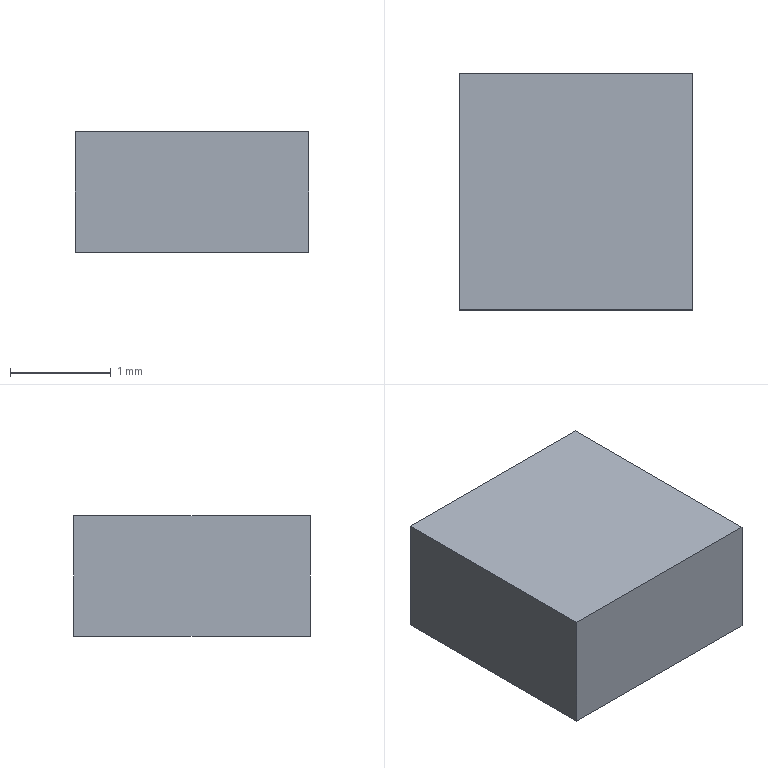Part | Creo | 1 solid | 6 faces | box 2.318 x 2.344 x 1.2 mm | volume 6.521 mm3 | plane 6
STEP:
#1=CARTESIAN_POINT('',(0.,0.,0.));
#2=DIRECTION('',(0.,0.,1.));
#3=DIRECTION('',(1.,0.,0.));
#4=AXIS2_PLACEMENT_3D('',#1,#2,#3);
#5=CARTESIAN_POINT('',(-1.125,-1.125,0.));
#6=VERTEX_POINT('',#5);
#7=CARTESIAN_POINT('',(1.193,-1.125,0.));
#8=VERTEX_POINT('',#7);
#9=CARTESIAN_POINT('',(-1.125,-1.125,0.));
#10=DIRECTION('',(1.,0.,0.));
#11=VECTOR('',#10,2.318);
#12=LINE('',#9,#11);
#13=EDGE_CURVE('',#6,#8,#12,.T.);
#14=ORIENTED_EDGE('',*,*,#13,.T.);
#15=CARTESIAN_POINT('',(1.193,1.219,0.));
#16=VERTEX_POINT('',#15);
#17=CARTESIAN_POINT('',(1.193,-1.125,0.));
#18=DIRECTION('',(0.,1.,0.));
#19=VECTOR('',#18,2.344);
#20=LINE('',#17,#19);
#21=EDGE_CURVE('',#8,#16,#20,.T.);
#22=ORIENTED_EDGE('',*,*,#21,.T.);
#23=CARTESIAN_POINT('',(-1.125,1.219,0.));
#24=VERTEX_POINT('',#23);
#25=CARTESIAN_POINT('',(1.193,1.219,0.));
#26=DIRECTION('',(-1.,0.,0.));
#27=VECTOR('',#26,2.318);
#28=LINE('',#25,#27);
#29=EDGE_CURVE('',#16,#24,#28,.T.);
#30=ORIENTED_EDGE('',*,*,#29,.T.);
#31=CARTESIAN_POINT('',(-1.125,1.219,0.));
#32=DIRECTION('',(0.,-1.,0.));
#33=VECTOR('',#32,2.344);
#34=LINE('',#31,#33);
#35=EDGE_CURVE('',#24,#6,#34,.T.);
#36=ORIENTED_EDGE('',*,*,#35,.T.);
#37=EDGE_LOOP('',(#14,#22,#30,#36));
#38=FACE_OUTER_BOUND('',#37,.F.);
#39=CARTESIAN_POINT('',(0.,0.,0.));
#40=DIRECTION('',(0.,0.,1.));
#41=DIRECTION('',(1.,0.,0.));
#42=AXIS2_PLACEMENT_3D('',#39,#40,#41);
#43=PLANE('',#42);
#44=ADVANCED_FACE('',(#38),#43,.F.);
#45=ORIENTED_EDGE('',*,*,#13,.F.);
#46=CARTESIAN_POINT('',(-1.125,-1.125,1.2));
#47=VERTEX_POINT('',#46);
#48=CARTESIAN_POINT('',(-1.125,-1.125,0.));
#49=DIRECTION('',(0.,0.,1.));
#50=VECTOR('',#49,1.2);
#51=LINE('',#48,#50);
#52=EDGE_CURVE('',#6,#47,#51,.T.);
#53=ORIENTED_EDGE('',*,*,#52,.T.);
#54=CARTESIAN_POINT('',(1.193,-1.125,1.2));
#55=VERTEX_POINT('',#54);
#56=CARTESIAN_POINT('',(-1.125,-1.125,1.2));
#57=DIRECTION('',(1.,0.,0.));
#58=VECTOR('',#57,2.318);
#59=LINE('',#56,#58);
#60=EDGE_CURVE('',#47,#55,#59,.T.);
#61=ORIENTED_EDGE('',*,*,#60,.T.);
#62=CARTESIAN_POINT('',(1.193,-1.125,0.));
#63=DIRECTION('',(0.,0.,1.));
#64=VECTOR('',#63,1.2);
#65=LINE('',#62,#64);
#66=EDGE_CURVE('',#8,#55,#65,.T.);
#67=ORIENTED_EDGE('',*,*,#66,.F.);
#68=EDGE_LOOP('',(#45,#53,#61,#67));
#69=FACE_OUTER_BOUND('',#68,.F.);
#70=CARTESIAN_POINT('',(-1.125,-1.125,0.));
#71=DIRECTION('',(0.,-1.,0.));
#72=DIRECTION('',(1.,0.,0.));
#73=AXIS2_PLACEMENT_3D('',#70,#71,#72);
#74=PLANE('',#73);
#75=ADVANCED_FACE('',(#69),#74,.T.);
#76=ORIENTED_EDGE('',*,*,#35,.F.);
#77=CARTESIAN_POINT('',(-1.125,1.219,1.2));
#78=VERTEX_POINT('',#77);
#79=CARTESIAN_POINT('',(-1.125,1.219,0.));
#80=DIRECTION('',(0.,0.,1.));
#81=VECTOR('',#80,1.2);
#82=LINE('',#79,#81);
#83=EDGE_CURVE('',#24,#78,#82,.T.);
#84=ORIENTED_EDGE('',*,*,#83,.T.);
#85=CARTESIAN_POINT('',(-1.125,1.219,1.2));
#86=DIRECTION('',(0.,-1.,0.));
#87=VECTOR('',#86,2.344);
#88=LINE('',#85,#87);
#89=EDGE_CURVE('',#78,#47,#88,.T.);
#90=ORIENTED_EDGE('',*,*,#89,.T.);
#91=ORIENTED_EDGE('',*,*,#52,.F.);
#92=EDGE_LOOP('',(#76,#84,#90,#91));
#93=FACE_OUTER_BOUND('',#92,.F.);
#94=CARTESIAN_POINT('',(-1.125,1.219,0.));
#95=DIRECTION('',(-1.,0.,0.));
#96=DIRECTION('',(0.,-1.,0.));
#97=AXIS2_PLACEMENT_3D('',#94,#95,#96);
#98=PLANE('',#97);
#99=ADVANCED_FACE('',(#93),#98,.T.);
#100=ORIENTED_EDGE('',*,*,#29,.F.);
#101=CARTESIAN_POINT('',(1.193,1.219,1.2));
#102=VERTEX_POINT('',#101);
#103=CARTESIAN_POINT('',(1.193,1.219,0.));
#104=DIRECTION('',(0.,0.,1.));
#105=VECTOR('',#104,1.2);
#106=LINE('',#103,#105);
#107=EDGE_CURVE('',#16,#102,#106,.T.);
#108=ORIENTED_EDGE('',*,*,#107,.T.);
#109=CARTESIAN_POINT('',(1.193,1.219,1.2));
#110=DIRECTION('',(-1.,0.,0.));
#111=VECTOR('',#110,2.318);
#112=LINE('',#109,#111);
#113=EDGE_CURVE('',#102,#78,#112,.T.);
#114=ORIENTED_EDGE('',*,*,#113,.T.);
#115=ORIENTED_EDGE('',*,*,#83,.F.);
#116=EDGE_LOOP('',(#100,#108,#114,#115));
#117=FACE_OUTER_BOUND('',#116,.F.);
#118=CARTESIAN_POINT('',(1.193,1.219,0.));
#119=DIRECTION('',(0.,1.,0.));
#120=DIRECTION('',(-1.,0.,0.));
#121=AXIS2_PLACEMENT_3D('',#118,#119,#120);
#122=PLANE('',#121);
#123=ADVANCED_FACE('',(#117),#122,.T.);
#124=ORIENTED_EDGE('',*,*,#21,.F.);
#125=ORIENTED_EDGE('',*,*,#66,.T.);
#126=CARTESIAN_POINT('',(1.193,-1.125,1.2));
#127=DIRECTION('',(0.,1.,0.));
#128=VECTOR('',#127,2.344);
#129=LINE('',#126,#128);
#130=EDGE_CURVE('',#55,#102,#129,.T.);
#131=ORIENTED_EDGE('',*,*,#130,.T.);
#132=ORIENTED_EDGE('',*,*,#107,.F.);
#133=EDGE_LOOP('',(#124,#125,#131,#132));
#134=FACE_OUTER_BOUND('',#133,.F.);
#135=CARTESIAN_POINT('',(1.193,-1.125,0.));
#136=DIRECTION('',(1.,0.,0.));
#137=DIRECTION('',(0.,1.,0.));
#138=AXIS2_PLACEMENT_3D('',#135,#136,#137);
#139=PLANE('',#138);
#140=ADVANCED_FACE('',(#134),#139,.T.);
#141=ORIENTED_EDGE('',*,*,#60,.F.);
#142=ORIENTED_EDGE('',*,*,#89,.F.);
#143=ORIENTED_EDGE('',*,*,#113,.F.);
#144=ORIENTED_EDGE('',*,*,#130,.F.);
#145=EDGE_LOOP('',(#141,#142,#143,#144));
#146=FACE_OUTER_BOUND('',#145,.F.);
#147=CARTESIAN_POINT('',(0.,0.,1.2));
#148=DIRECTION('',(0.,0.,1.));
#149=DIRECTION('',(1.,0.,0.));
#150=AXIS2_PLACEMENT_3D('',#147,#148,#149);
#151=PLANE('',#150);
#152=ADVANCED_FACE('',(#146),#151,.T.);
#153=CLOSED_SHELL('',(#44,#75,#99,#123,#140,#152));
#154=MANIFOLD_SOLID_BREP('',#153);
#155=(LENGTH_UNIT()NAMED_UNIT(*)SI_UNIT(.MILLI.,.METRE.));
#156=UNCERTAINTY_MEASURE_WITH_UNIT(LENGTH_MEASURE(0.0003508),#155,'','');
#157=(NAMED_UNIT(*)PLANE_ANGLE_UNIT()SI_UNIT($,.RADIAN.));
#158=PLANE_ANGLE_MEASURE_WITH_UNIT(PLANE_ANGLE_MEASURE(0.01745),#157);
#159=(CONVERSION_BASED_UNIT('DEGREE',#158)NAMED_UNIT(*)PLANE_ANGLE_UNIT());
#160=(NAMED_UNIT(*)SI_UNIT($,.STERADIAN.)SOLID_ANGLE_UNIT());
#161=(GEOMETRIC_REPRESENTATION_CONTEXT(3)GLOBAL_UNCERTAINTY_ASSIGNED_CONTEXT((#156))GLOBAL_UNIT_ASSIGNED_CONTEXT((#155,#159,#160))REPRESENTATION_CONTEXT('',''));
#162=ADVANCED_BREP_SHAPE_REPRESENTATION('',(#4,#154),#161);